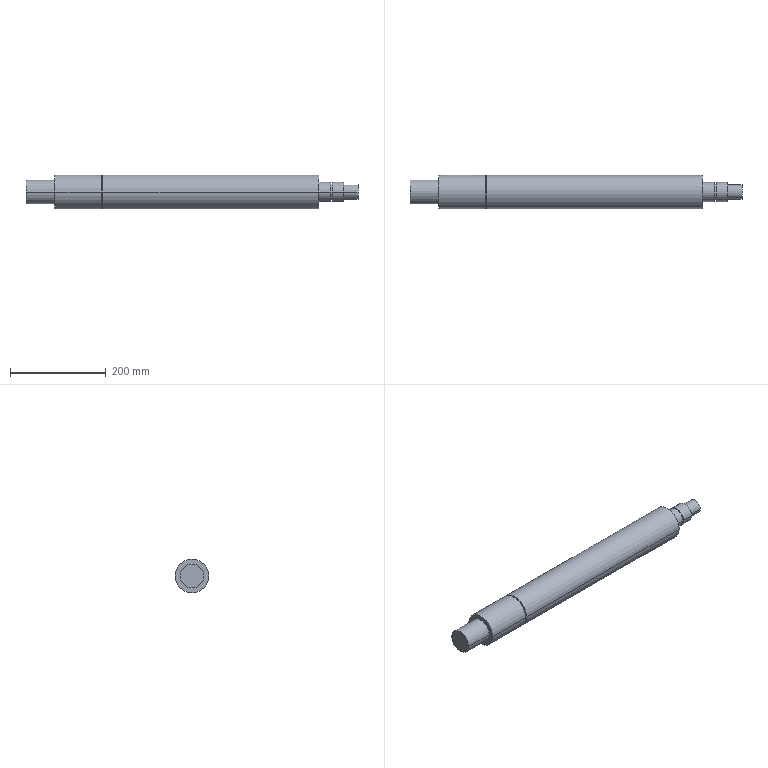Part | SolidWorks | features ICE 1, Revolution 1 | 1 solid | 30 faces | box 691.99 x 70 x 70 mm | volume 2315644 mm3 | cylinder 18 | plane 12 | commonest cylinder face diameters 40 x4 70 x4 12 x2 30 x2 34.7 x2 50 x2
STEP:
#1=CARTESIAN_POINT('',(691.99,-15.,0.));
#2=VERTEX_POINT('',#1);
#3=CARTESIAN_POINT('',(691.99,15.,0.));
#4=VERTEX_POINT('',#3);
#5=CARTESIAN_POINT('',(691.99,0.,0.));
#6=DIRECTION('',(-1.,0.,0.));
#7=DIRECTION('',(0.,-1.,0.));
#8=AXIS2_PLACEMENT_3D('',#5,#6,#7);
#9=CIRCLE('',#8,15.);
#10=EDGE_CURVE('',#2,#4,#9,.T.);
#11=ORIENTED_EDGE('',*,*,#10,.T.);
#12=CARTESIAN_POINT('',(661.99,15.,0.));
#13=VERTEX_POINT('',#12);
#14=CARTESIAN_POINT('',(0.,15.,0.));
#15=DIRECTION('',(-1.,0.,0.));
#16=VECTOR('',#15,1000.);
#17=LINE('',#14,#16);
#18=EDGE_CURVE('',#4,#13,#17,.T.);
#19=ORIENTED_EDGE('',*,*,#18,.T.);
#20=CARTESIAN_POINT('',(661.99,-15.,0.));
#21=VERTEX_POINT('',#20);
#22=CARTESIAN_POINT('',(661.99,0.,0.));
#23=DIRECTION('',(-1.,0.,0.));
#24=DIRECTION('',(0.,-1.,0.));
#25=AXIS2_PLACEMENT_3D('',#22,#23,#24);
#26=CIRCLE('',#25,15.);
#27=EDGE_CURVE('',#21,#13,#26,.T.);
#28=ORIENTED_EDGE('',*,*,#27,.F.);
#29=CARTESIAN_POINT('',(0.,-15.,0.));
#30=DIRECTION('',(-1.,0.,0.));
#31=VECTOR('',#30,1000.);
#32=LINE('',#29,#31);
#33=EDGE_CURVE('',#2,#21,#32,.T.);
#34=ORIENTED_EDGE('',*,*,#33,.F.);
#35=EDGE_LOOP('',(#11,#19,#28,#34));
#36=FACE_OUTER_BOUND('',#35,.T.);
#37=CARTESIAN_POINT('',(0.,0.,0.));
#38=DIRECTION('',(-1.,0.,0.));
#39=DIRECTION('',(0.,-1.,0.));
#40=AXIS2_PLACEMENT_3D('',#37,#38,#39);
#41=CYLINDRICAL_SURFACE('',#40,15.);
#42=ADVANCED_FACE('',(#36),#41,.T.);
#43=CARTESIAN_POINT('',(661.99,-20.,0.));
#44=VERTEX_POINT('',#43);
#45=CARTESIAN_POINT('',(661.99,20.,0.));
#46=VERTEX_POINT('',#45);
#47=CARTESIAN_POINT('',(661.99,0.,0.));
#48=DIRECTION('',(-1.,0.,0.));
#49=DIRECTION('',(0.,-1.,0.));
#50=AXIS2_PLACEMENT_3D('',#47,#48,#49);
#51=CIRCLE('',#50,20.);
#52=EDGE_CURVE('',#44,#46,#51,.T.);
#53=ORIENTED_EDGE('',*,*,#52,.T.);
#54=CARTESIAN_POINT('',(638.32,20.,0.));
#55=VERTEX_POINT('',#54);
#56=CARTESIAN_POINT('',(0.,20.,0.));
#57=DIRECTION('',(-1.,0.,0.));
#58=VECTOR('',#57,1000.);
#59=LINE('',#56,#58);
#60=EDGE_CURVE('',#46,#55,#59,.T.);
#61=ORIENTED_EDGE('',*,*,#60,.T.);
#62=CARTESIAN_POINT('',(638.32,-20.,0.));
#63=VERTEX_POINT('',#62);
#64=CARTESIAN_POINT('',(638.32,0.,0.));
#65=DIRECTION('',(-1.,0.,0.));
#66=DIRECTION('',(0.,-1.,0.));
#67=AXIS2_PLACEMENT_3D('',#64,#65,#66);
#68=CIRCLE('',#67,20.);
#69=EDGE_CURVE('',#63,#55,#68,.T.);
#70=ORIENTED_EDGE('',*,*,#69,.F.);
#71=CARTESIAN_POINT('',(0.,-20.,0.));
#72=DIRECTION('',(-1.,0.,0.));
#73=VECTOR('',#72,1000.);
#74=LINE('',#71,#73);
#75=EDGE_CURVE('',#44,#63,#74,.T.);
#76=ORIENTED_EDGE('',*,*,#75,.F.);
#77=EDGE_LOOP('',(#53,#61,#70,#76));
#78=FACE_OUTER_BOUND('',#77,.T.);
#79=CARTESIAN_POINT('',(0.,0.,0.));
#80=DIRECTION('',(-1.,0.,0.));
#81=DIRECTION('',(0.,-1.,0.));
#82=AXIS2_PLACEMENT_3D('',#79,#80,#81);
#83=CYLINDRICAL_SURFACE('',#82,20.);
#84=ADVANCED_FACE('',(#78),#83,.T.);
#85=CARTESIAN_POINT('',(638.32,-17.35,0.));
#86=VERTEX_POINT('',#85);
#87=CARTESIAN_POINT('',(638.32,17.35,0.));
#88=VERTEX_POINT('',#87);
#89=CARTESIAN_POINT('',(638.32,0.,0.));
#90=DIRECTION('',(-1.,0.,0.));
#91=DIRECTION('',(0.,-1.,0.));
#92=AXIS2_PLACEMENT_3D('',#89,#90,#91);
#93=CIRCLE('',#92,17.35);
#94=EDGE_CURVE('',#86,#88,#93,.T.);
#95=ORIENTED_EDGE('',*,*,#94,.T.);
#96=CARTESIAN_POINT('',(635.67,17.35,0.));
#97=VERTEX_POINT('',#96);
#98=CARTESIAN_POINT('',(0.,17.35,0.));
#99=DIRECTION('',(-1.,0.,0.));
#100=VECTOR('',#99,1000.);
#101=LINE('',#98,#100);
#102=EDGE_CURVE('',#88,#97,#101,.T.);
#103=ORIENTED_EDGE('',*,*,#102,.T.);
#104=CARTESIAN_POINT('',(635.67,-17.35,0.));
#105=VERTEX_POINT('',#104);
#106=CARTESIAN_POINT('',(635.67,0.,0.));
#107=DIRECTION('',(-1.,0.,0.));
#108=DIRECTION('',(0.,-1.,0.));
#109=AXIS2_PLACEMENT_3D('',#106,#107,#108);
#110=CIRCLE('',#109,17.35);
#111=EDGE_CURVE('',#105,#97,#110,.T.);
#112=ORIENTED_EDGE('',*,*,#111,.F.);
#113=CARTESIAN_POINT('',(0.,-17.35,0.));
#114=DIRECTION('',(-1.,0.,0.));
#115=VECTOR('',#114,1000.);
#116=LINE('',#113,#115);
#117=EDGE_CURVE('',#86,#105,#116,.T.);
#118=ORIENTED_EDGE('',*,*,#117,.F.);
#119=EDGE_LOOP('',(#95,#103,#112,#118));
#120=FACE_OUTER_BOUND('',#119,.T.);
#121=CARTESIAN_POINT('',(0.,0.,0.));
#122=DIRECTION('',(-1.,0.,0.));
#123=DIRECTION('',(0.,-1.,0.));
#124=AXIS2_PLACEMENT_3D('',#121,#122,#123);
#125=CYLINDRICAL_SURFACE('',#124,17.35);
#126=ADVANCED_FACE('',(#120),#125,.T.);
#127=CARTESIAN_POINT('',(635.67,-20.,0.));
#128=VERTEX_POINT('',#127);
#129=CARTESIAN_POINT('',(635.67,20.,0.));
#130=VERTEX_POINT('',#129);
#131=CARTESIAN_POINT('',(635.67,0.,0.));
#132=DIRECTION('',(-1.,0.,0.));
#133=DIRECTION('',(0.,-1.,0.));
#134=AXIS2_PLACEMENT_3D('',#131,#132,#133);
#135=CIRCLE('',#134,20.);
#136=EDGE_CURVE('',#128,#130,#135,.T.);
#137=ORIENTED_EDGE('',*,*,#136,.T.);
#138=CARTESIAN_POINT('',(610.,20.,0.));
#139=VERTEX_POINT('',#138);
#140=CARTESIAN_POINT('',(0.,20.,0.));
#141=DIRECTION('',(-1.,0.,0.));
#142=VECTOR('',#141,1000.);
#143=LINE('',#140,#142);
#144=EDGE_CURVE('',#130,#139,#143,.T.);
#145=ORIENTED_EDGE('',*,*,#144,.T.);
#146=CARTESIAN_POINT('',(610.,-20.,0.));
#147=VERTEX_POINT('',#146);
#148=CARTESIAN_POINT('',(610.,0.,0.));
#149=DIRECTION('',(-1.,0.,0.));
#150=DIRECTION('',(0.,-1.,0.));
#151=AXIS2_PLACEMENT_3D('',#148,#149,#150);
#152=CIRCLE('',#151,20.);
#153=EDGE_CURVE('',#147,#139,#152,.T.);
#154=ORIENTED_EDGE('',*,*,#153,.F.);
#155=CARTESIAN_POINT('',(0.,-20.,0.));
#156=DIRECTION('',(-1.,0.,0.));
#157=VECTOR('',#156,1000.);
#158=LINE('',#155,#157);
#159=EDGE_CURVE('',#128,#147,#158,.T.);
#160=ORIENTED_EDGE('',*,*,#159,.F.);
#161=EDGE_LOOP('',(#137,#145,#154,#160));
#162=FACE_OUTER_BOUND('',#161,.T.);
#163=CARTESIAN_POINT('',(0.,0.,0.));
#164=DIRECTION('',(-1.,0.,0.));
#165=DIRECTION('',(0.,-1.,0.));
#166=AXIS2_PLACEMENT_3D('',#163,#164,#165);
#167=CYLINDRICAL_SURFACE('',#166,20.);
#168=ADVANCED_FACE('',(#162),#167,.T.);
#169=CARTESIAN_POINT('',(610.,-35.,0.));
#170=VERTEX_POINT('',#169);
#171=CARTESIAN_POINT('',(610.,35.,0.));
#172=VERTEX_POINT('',#171);
#173=CARTESIAN_POINT('',(610.,0.,0.));
#174=DIRECTION('',(-1.,0.,0.));
#175=DIRECTION('',(0.,-1.,0.));
#176=AXIS2_PLACEMENT_3D('',#173,#174,#175);
#177=CIRCLE('',#176,35.);
#178=EDGE_CURVE('',#170,#172,#177,.T.);
#179=ORIENTED_EDGE('',*,*,#178,.T.);
#180=CARTESIAN_POINT('',(160.,35.,0.));
#181=VERTEX_POINT('',#180);
#182=CARTESIAN_POINT('',(0.,35.,0.));
#183=DIRECTION('',(-1.,0.,0.));
#184=VECTOR('',#183,1000.);
#185=LINE('',#182,#184);
#186=EDGE_CURVE('',#172,#181,#185,.T.);
#187=ORIENTED_EDGE('',*,*,#186,.T.);
#188=CARTESIAN_POINT('',(160.,-35.,0.));
#189=VERTEX_POINT('',#188);
#190=CARTESIAN_POINT('',(160.,0.,0.));
#191=DIRECTION('',(-1.,0.,0.));
#192=DIRECTION('',(0.,-1.,0.));
#193=AXIS2_PLACEMENT_3D('',#190,#191,#192);
#194=CIRCLE('',#193,35.);
#195=EDGE_CURVE('',#189,#181,#194,.T.);
#196=ORIENTED_EDGE('',*,*,#195,.F.);
#197=CARTESIAN_POINT('',(0.,-35.,0.));
#198=DIRECTION('',(-1.,0.,0.));
#199=VECTOR('',#198,1000.);
#200=LINE('',#197,#199);
#201=EDGE_CURVE('',#170,#189,#200,.T.);
#202=ORIENTED_EDGE('',*,*,#201,.F.);
#203=EDGE_LOOP('',(#179,#187,#196,#202));
#204=FACE_OUTER_BOUND('',#203,.T.);
#205=CARTESIAN_POINT('',(0.,0.,0.));
#206=DIRECTION('',(-1.,0.,0.));
#207=DIRECTION('',(0.,-1.,0.));
#208=AXIS2_PLACEMENT_3D('',#205,#206,#207);
#209=CYLINDRICAL_SURFACE('',#208,35.);
#210=ADVANCED_FACE('',(#204),#209,.T.);
#211=CARTESIAN_POINT('',(160.,-32.35,0.));
#212=VERTEX_POINT('',#211);
#213=CARTESIAN_POINT('',(160.,32.35,0.));
#214=VERTEX_POINT('',#213);
#215=CARTESIAN_POINT('',(160.,0.,0.));
#216=DIRECTION('',(-1.,0.,0.));
#217=DIRECTION('',(0.,-1.,0.));
#218=AXIS2_PLACEMENT_3D('',#215,#216,#217);
#219=CIRCLE('',#218,32.35);
#220=EDGE_CURVE('',#212,#214,#219,.T.);
#221=ORIENTED_EDGE('',*,*,#220,.T.);
#222=CARTESIAN_POINT('',(157.35,32.35,0.));
#223=VERTEX_POINT('',#222);
#224=CARTESIAN_POINT('',(0.,32.35,0.));
#225=DIRECTION('',(-1.,0.,0.));
#226=VECTOR('',#225,1000.);
#227=LINE('',#224,#226);
#228=EDGE_CURVE('',#214,#223,#227,.T.);
#229=ORIENTED_EDGE('',*,*,#228,.T.);
#230=CARTESIAN_POINT('',(157.35,-32.35,0.));
#231=VERTEX_POINT('',#230);
#232=CARTESIAN_POINT('',(157.35,0.,0.));
#233=DIRECTION('',(-1.,0.,0.));
#234=DIRECTION('',(0.,-1.,0.));
#235=AXIS2_PLACEMENT_3D('',#232,#233,#234);
#236=CIRCLE('',#235,32.35);
#237=EDGE_CURVE('',#231,#223,#236,.T.);
#238=ORIENTED_EDGE('',*,*,#237,.F.);
#239=CARTESIAN_POINT('',(0.,-32.35,0.));
#240=DIRECTION('',(-1.,0.,0.));
#241=VECTOR('',#240,1000.);
#242=LINE('',#239,#241);
#243=EDGE_CURVE('',#212,#231,#242,.T.);
#244=ORIENTED_EDGE('',*,*,#243,.F.);
#245=EDGE_LOOP('',(#221,#229,#238,#244));
#246=FACE_OUTER_BOUND('',#245,.T.);
#247=CARTESIAN_POINT('',(0.,0.,0.));
#248=DIRECTION('',(-1.,0.,0.));
#249=DIRECTION('',(0.,-1.,0.));
#250=AXIS2_PLACEMENT_3D('',#247,#248,#249);
#251=CYLINDRICAL_SURFACE('',#250,32.35);
#252=ADVANCED_FACE('',(#246),#251,.T.);
#253=CARTESIAN_POINT('',(60.,-25.,0.));
#254=VERTEX_POINT('',#253);
#255=CARTESIAN_POINT('',(60.,25.,0.));
#256=VERTEX_POINT('',#255);
#257=CARTESIAN_POINT('',(60.,0.,0.));
#258=DIRECTION('',(-1.,0.,0.));
#259=DIRECTION('',(0.,-1.,0.));
#260=AXIS2_PLACEMENT_3D('',#257,#258,#259);
#261=CIRCLE('',#260,25.);
#262=EDGE_CURVE('',#254,#256,#261,.T.);
#263=ORIENTED_EDGE('',*,*,#262,.T.);
#264=CARTESIAN_POINT('',(0.,25.,0.));
#265=VERTEX_POINT('',#264);
#266=CARTESIAN_POINT('',(0.,25.,0.));
#267=DIRECTION('',(-1.,0.,0.));
#268=VECTOR('',#267,1000.);
#269=LINE('',#266,#268);
#270=EDGE_CURVE('',#256,#265,#269,.T.);
#271=ORIENTED_EDGE('',*,*,#270,.T.);
#272=CARTESIAN_POINT('',(0.,-25.,0.));
#273=VERTEX_POINT('',#272);
#274=CARTESIAN_POINT('',(0.,0.,0.));
#275=DIRECTION('',(-1.,0.,0.));
#276=DIRECTION('',(0.,-1.,0.));
#277=AXIS2_PLACEMENT_3D('',#274,#275,#276);
#278=CIRCLE('',#277,25.);
#279=EDGE_CURVE('',#273,#265,#278,.T.);
#280=ORIENTED_EDGE('',*,*,#279,.F.);
#281=CARTESIAN_POINT('',(0.,-25.,0.));
#282=DIRECTION('',(-1.,0.,0.));
#283=VECTOR('',#282,1000.);
#284=LINE('',#281,#283);
#285=EDGE_CURVE('',#254,#273,#284,.T.);
#286=ORIENTED_EDGE('',*,*,#285,.F.);
#287=EDGE_LOOP('',(#263,#271,#280,#286));
#288=FACE_OUTER_BOUND('',#287,.T.);
#289=CARTESIAN_POINT('',(0.,0.,0.));
#290=DIRECTION('',(-1.,0.,0.));
#291=DIRECTION('',(0.,-1.,0.));
#292=AXIS2_PLACEMENT_3D('',#289,#290,#291);
#293=CYLINDRICAL_SURFACE('',#292,25.);
#294=ADVANCED_FACE('',(#288),#293,.T.);
#295=CARTESIAN_POINT('',(157.35,-35.,0.));
#296=VERTEX_POINT('',#295);
#297=CARTESIAN_POINT('',(157.35,35.,0.));
#298=VERTEX_POINT('',#297);
#299=CARTESIAN_POINT('',(157.35,0.,0.));
#300=DIRECTION('',(-1.,0.,0.));
#301=DIRECTION('',(0.,-1.,0.));
#302=AXIS2_PLACEMENT_3D('',#299,#300,#301);
#303=CIRCLE('',#302,35.);
#304=EDGE_CURVE('',#296,#298,#303,.T.);
#305=ORIENTED_EDGE('',*,*,#304,.T.);
#306=CARTESIAN_POINT('',(130.,35.,0.));
#307=VERTEX_POINT('',#306);
#308=CARTESIAN_POINT('',(0.,35.,0.));
#309=DIRECTION('',(-1.,0.,0.));
#310=VECTOR('',#309,1000.);
#311=LINE('',#308,#310);
#312=EDGE_CURVE('',#298,#307,#311,.T.);
#313=ORIENTED_EDGE('',*,*,#312,.T.);
#314=CARTESIAN_POINT('',(124.,34.482,6.));
#315=VERTEX_POINT('',#314);
#316=CARTESIAN_POINT('',(124.,34.482,6.));
#317=CARTESIAN_POINT('',(124.397,34.482,6.));
#318=CARTESIAN_POINT('',(124.788,34.489,5.961));
#319=CARTESIAN_POINT('',(125.364,34.508,5.846));
#320=CARTESIAN_POINT('',(125.554,34.516,5.799));
#321=CARTESIAN_POINT('',(125.932,34.535,5.684));
#322=CARTESIAN_POINT('',(126.119,34.546,5.617));
#323=CARTESIAN_POINT('',(126.664,34.583,5.391));
#324=CARTESIAN_POINT('',(127.008,34.611,5.206));
#325=CARTESIAN_POINT('',(127.66,34.674,4.77));
#326=CARTESIAN_POINT('',(127.968,34.708,4.517));
#327=CARTESIAN_POINT('',(128.521,34.776,3.965));
#328=CARTESIAN_POINT('',(128.769,34.809,3.663));
#329=CARTESIAN_POINT('',(129.207,34.872,3.007));
#330=CARTESIAN_POINT('',(129.393,34.901,2.659));
#331=CARTESIAN_POINT('',(129.618,34.936,2.117));
#332=CARTESIAN_POINT('',(129.684,34.947,1.933));
#333=CARTESIAN_POINT('',(129.798,34.966,1.557));
#334=CARTESIAN_POINT('',(129.846,34.974,1.364));
#335=CARTESIAN_POINT('',(129.962,34.993,0.7822));
#336=CARTESIAN_POINT('',(130.,35.,0.3923));
#337=CARTESIAN_POINT('',(130.,35.,0.));
#338=B_SPLINE_CURVE_WITH_KNOTS('',3,(#316,#317,#318,#319,#320,#321,#322,#323,#324,#325,#326,#327,#328,#329,#330,#331,#332,#333,#334,#335,#336,#337),.UNSPECIFIED.,.F.,.F.,(4,2,2,2,2,2,2,2,2,2,4),(0.,0.001175,0.001762,0.00235,0.003525,0.004699,0.005874,0.007049,0.007637,0.008224,0.009399),.UNSPECIFIED.);
#339=EDGE_CURVE('',#315,#307,#338,.T.);
#340=ORIENTED_EDGE('',*,*,#339,.F.);
#341=CARTESIAN_POINT('',(81.,34.482,6.));
#342=VERTEX_POINT('',#341);
#343=CARTESIAN_POINT('',(0.,34.482,6.));
#344=DIRECTION('',(1.,0.,0.));
#345=VECTOR('',#344,1000.);
#346=LINE('',#343,#345);
#347=EDGE_CURVE('',#342,#315,#346,.T.);
#348=ORIENTED_EDGE('',*,*,#347,.F.);
#349=CARTESIAN_POINT('',(75.,35.,0.));
#350=VERTEX_POINT('',#349);
#351=CARTESIAN_POINT('',(75.,35.,0.));
#352=CARTESIAN_POINT('',(75.,35.,0.3919));
#353=CARTESIAN_POINT('',(75.039,34.993,0.79));
#354=CARTESIAN_POINT('',(75.193,34.967,1.559));
#355=CARTESIAN_POINT('',(75.306,34.948,1.934));
#356=CARTESIAN_POINT('',(75.532,34.913,2.479));
#357=CARTESIAN_POINT('',(75.617,34.899,2.658));
#358=CARTESIAN_POINT('',(75.803,34.871,3.005));
#359=CARTESIAN_POINT('',(75.904,34.856,3.173));
#360=CARTESIAN_POINT('',(76.229,34.81,3.659));
#361=CARTESIAN_POINT('',(76.478,34.776,3.963));
#362=CARTESIAN_POINT('',(77.036,34.708,4.521));
#363=CARTESIAN_POINT('',(77.338,34.674,4.769));
#364=CARTESIAN_POINT('',(77.824,34.627,5.094));
#365=CARTESIAN_POINT('',(77.992,34.612,5.195));
#366=CARTESIAN_POINT('',(78.339,34.584,5.381));
#367=CARTESIAN_POINT('',(78.518,34.571,5.466));
#368=CARTESIAN_POINT('',(79.062,34.534,5.692));
#369=CARTESIAN_POINT('',(79.436,34.515,5.806));
#370=CARTESIAN_POINT('',(80.206,34.489,5.96));
#371=CARTESIAN_POINT('',(80.603,34.482,6.));
#372=CARTESIAN_POINT('',(81.,34.482,6.));
#373=B_SPLINE_CURVE_WITH_KNOTS('',3,(#351,#352,#353,#354,#355,#356,#357,#358,#359,#360,#361,#362,#363,#364,#365,#366,#367,#368,#369,#370,#371,#372),.UNSPECIFIED.,.F.,.F.,(4,2,2,2,2,2,2,2,2,2,4),(0.009399,0.01057,0.01175,0.01233,0.01292,0.01409,0.01527,0.01585,0.01644,0.01761,0.01879),.UNSPECIFIED.);
#374=EDGE_CURVE('',#350,#342,#373,.T.);
#375=ORIENTED_EDGE('',*,*,#374,.F.);
#376=CARTESIAN_POINT('',(60.,35.,0.));
#377=VERTEX_POINT('',#376);
#378=CARTESIAN_POINT('',(0.,35.,0.));
#379=DIRECTION('',(-1.,0.,0.));
#380=VECTOR('',#379,1000.);
#381=LINE('',#378,#380);
#382=EDGE_CURVE('',#350,#377,#381,.T.);
#383=ORIENTED_EDGE('',*,*,#382,.T.);
#384=CARTESIAN_POINT('',(60.,-35.,0.));
#385=VERTEX_POINT('',#384);
#386=CARTESIAN_POINT('',(60.,0.,0.));
#387=DIRECTION('',(-1.,0.,0.));
#388=DIRECTION('',(0.,-1.,0.));
#389=AXIS2_PLACEMENT_3D('',#386,#387,#388);
#390=CIRCLE('',#389,35.);
#391=EDGE_CURVE('',#385,#377,#390,.T.);
#392=ORIENTED_EDGE('',*,*,#391,.F.);
#393=CARTESIAN_POINT('',(0.,-35.,0.));
#394=DIRECTION('',(-1.,0.,0.));
#395=VECTOR('',#394,1000.);
#396=LINE('',#393,#395);
#397=EDGE_CURVE('',#296,#385,#396,.T.);
#398=ORIENTED_EDGE('',*,*,#397,.F.);
#399=EDGE_LOOP('',(#305,#313,#340,#348,#375,#383,#392,#398));
#400=FACE_OUTER_BOUND('',#399,.T.);
#401=CARTESIAN_POINT('',(0.,0.,0.));
#402=DIRECTION('',(-1.,0.,0.));
#403=DIRECTION('',(0.,-1.,0.));
#404=AXIS2_PLACEMENT_3D('',#401,#402,#403);
#405=CYLINDRICAL_SURFACE('',#404,35.);
#406=ADVANCED_FACE('',(#400),#405,.T.);
#407=ORIENTED_EDGE('',*,*,#312,.F.);
#408=CARTESIAN_POINT('',(157.35,0.,0.));
#409=DIRECTION('',(-1.,0.,0.));
#410=DIRECTION('',(0.,-1.,0.));
#411=AXIS2_PLACEMENT_3D('',#408,#409,#410);
#412=CIRCLE('',#411,35.);
#413=EDGE_CURVE('',#298,#296,#412,.T.);
#414=ORIENTED_EDGE('',*,*,#413,.T.);
#415=ORIENTED_EDGE('',*,*,#397,.T.);
#416=CARTESIAN_POINT('',(60.,0.,0.));
#417=DIRECTION('',(-1.,0.,0.));
#418=DIRECTION('',(0.,-1.,0.));
#419=AXIS2_PLACEMENT_3D('',#416,#417,#418);
#420=CIRCLE('',#419,35.);
#421=EDGE_CURVE('',#377,#385,#420,.T.);
#422=ORIENTED_EDGE('',*,*,#421,.F.);
#423=ORIENTED_EDGE('',*,*,#382,.F.);
#424=CARTESIAN_POINT('',(81.,34.482,-6.));
#425=VERTEX_POINT('',#424);
#426=CARTESIAN_POINT('',(81.,34.482,-6.));
#427=CARTESIAN_POINT('',(80.603,34.482,-6.));
#428=CARTESIAN_POINT('',(80.212,34.489,-5.961));
#429=CARTESIAN_POINT('',(79.636,34.508,-5.846));
#430=CARTESIAN_POINT('',(79.446,34.516,-5.799));
#431=CARTESIAN_POINT('',(79.068,34.535,-5.684));
#432=CARTESIAN_POINT('',(78.881,34.546,-5.617));
#433=CARTESIAN_POINT('',(78.336,34.583,-5.391));
#434=CARTESIAN_POINT('',(77.992,34.611,-5.206));
#435=CARTESIAN_POINT('',(77.34,34.674,-4.77));
#436=CARTESIAN_POINT('',(77.032,34.708,-4.517));
#437=CARTESIAN_POINT('',(76.479,34.776,-3.965));
#438=CARTESIAN_POINT('',(76.231,34.809,-3.663));
#439=CARTESIAN_POINT('',(75.793,34.872,-3.007));
#440=CARTESIAN_POINT('',(75.607,34.901,-2.659));
#441=CARTESIAN_POINT('',(75.382,34.936,-2.117));
#442=CARTESIAN_POINT('',(75.316,34.947,-1.933));
#443=CARTESIAN_POINT('',(75.202,34.966,-1.557));
#444=CARTESIAN_POINT('',(75.154,34.974,-1.364));
#445=CARTESIAN_POINT('',(75.038,34.993,-0.7822));
#446=CARTESIAN_POINT('',(75.,35.,-0.3923));
#447=CARTESIAN_POINT('',(75.,35.,0.));
#448=B_SPLINE_CURVE_WITH_KNOTS('',3,(#426,#427,#428,#429,#430,#431,#432,#433,#434,#435,#436,#437,#438,#439,#440,#441,#442,#443,#444,#445,#446,#447),.UNSPECIFIED.,.F.,.F.,(4,2,2,2,2,2,2,2,2,2,4),(0.,0.001175,0.001762,0.00235,0.003525,0.004699,0.005874,0.007049,0.007637,0.008224,0.009399),.UNSPECIFIED.);
#449=EDGE_CURVE('',#425,#350,#448,.T.);
#450=ORIENTED_EDGE('',*,*,#449,.F.);
#451=CARTESIAN_POINT('',(124.,34.482,-6.));
#452=VERTEX_POINT('',#451);
#453=CARTESIAN_POINT('',(0.,34.482,-6.));
#454=DIRECTION('',(-1.,0.,0.));
#455=VECTOR('',#454,1000.);
#456=LINE('',#453,#455);
#457=EDGE_CURVE('',#452,#425,#456,.T.);
#458=ORIENTED_EDGE('',*,*,#457,.F.);
#459=CARTESIAN_POINT('',(130.,35.,0.));
#460=CARTESIAN_POINT('',(130.,35.,-0.3919));
#461=CARTESIAN_POINT('',(129.961,34.993,-0.79));
#462=CARTESIAN_POINT('',(129.807,34.967,-1.559));
#463=CARTESIAN_POINT('',(129.694,34.948,-1.934));
#464=CARTESIAN_POINT('',(129.468,34.913,-2.479));
#465=CARTESIAN_POINT('',(129.383,34.899,-2.658));
#466=CARTESIAN_POINT('',(129.197,34.871,-3.005));
#467=CARTESIAN_POINT('',(129.096,34.856,-3.173));
#468=CARTESIAN_POINT('',(128.771,34.81,-3.659));
#469=CARTESIAN_POINT('',(128.522,34.776,-3.963));
#470=CARTESIAN_POINT('',(127.964,34.708,-4.521));
#471=CARTESIAN_POINT('',(127.662,34.674,-4.769));
#472=CARTESIAN_POINT('',(127.176,34.627,-5.094));
#473=CARTESIAN_POINT('',(127.008,34.612,-5.195));
#474=CARTESIAN_POINT('',(126.661,34.584,-5.381));
#475=CARTESIAN_POINT('',(126.482,34.571,-5.466));
#476=CARTESIAN_POINT('',(125.938,34.534,-5.692));
#477=CARTESIAN_POINT('',(125.564,34.515,-5.806));
#478=CARTESIAN_POINT('',(124.794,34.489,-5.96));
#479=CARTESIAN_POINT('',(124.397,34.482,-6.));
#480=CARTESIAN_POINT('',(124.,34.482,-6.));
#481=B_SPLINE_CURVE_WITH_KNOTS('',3,(#459,#460,#461,#462,#463,#464,#465,#466,#467,#468,#469,#470,#471,#472,#473,#474,#475,#476,#477,#478,#479,#480),.UNSPECIFIED.,.F.,.F.,(4,2,2,2,2,2,2,2,2,2,4),(0.009399,0.01057,0.01175,0.01233,0.01292,0.01409,0.01527,0.01585,0.01644,0.01761,0.01879),.UNSPECIFIED.);
#482=EDGE_CURVE('',#307,#452,#481,.T.);
#483=ORIENTED_EDGE('',*,*,#482,.F.);
#484=EDGE_LOOP('',(#407,#414,#415,#422,#423,#450,#458,#483));
#485=FACE_OUTER_BOUND('',#484,.T.);
#486=CARTESIAN_POINT('',(0.,0.,0.));
#487=DIRECTION('',(-1.,0.,0.));
#488=DIRECTION('',(0.,-1.,0.));
#489=AXIS2_PLACEMENT_3D('',#486,#487,#488);
#490=CYLINDRICAL_SURFACE('',#489,35.);
#491=ADVANCED_FACE('',(#485),#490,.T.);
#492=ORIENTED_EDGE('',*,*,#279,.T.);
#493=CARTESIAN_POINT('',(0.,0.,0.));
#494=DIRECTION('',(-1.,0.,0.));
#495=DIRECTION('',(0.,-1.,0.));
#496=AXIS2_PLACEMENT_3D('',#493,#494,#495);
#497=CIRCLE('',#496,25.);
#498=EDGE_CURVE('',#265,#273,#497,.T.);
#499=ORIENTED_EDGE('',*,*,#498,.T.);
#500=EDGE_LOOP('',(#492,#499));
#501=FACE_OUTER_BOUND('',#500,.T.);
#502=CARTESIAN_POINT('',(0.,0.,0.));
#503=DIRECTION('',(1.,0.,0.));
#504=DIRECTION('',(0.,1.,0.));
#505=AXIS2_PLACEMENT_3D('',#502,#503,#504);
#506=PLANE('',#505);
#507=ADVANCED_FACE('',(#501),#506,.F.);
#508=ORIENTED_EDGE('',*,*,#270,.F.);
#509=CARTESIAN_POINT('',(60.,0.,0.));
#510=DIRECTION('',(-1.,0.,0.));
#511=DIRECTION('',(0.,-1.,0.));
#512=AXIS2_PLACEMENT_3D('',#509,#510,#511);
#513=CIRCLE('',#512,25.);
#514=EDGE_CURVE('',#256,#254,#513,.T.);
#515=ORIENTED_EDGE('',*,*,#514,.T.);
#516=ORIENTED_EDGE('',*,*,#285,.T.);
#517=ORIENTED_EDGE('',*,*,#498,.F.);
#518=EDGE_LOOP('',(#508,#515,#516,#517));
#519=FACE_OUTER_BOUND('',#518,.T.);
#520=CARTESIAN_POINT('',(0.,0.,0.));
#521=DIRECTION('',(-1.,0.,0.));
#522=DIRECTION('',(0.,-1.,0.));
#523=AXIS2_PLACEMENT_3D('',#520,#521,#522);
#524=CYLINDRICAL_SURFACE('',#523,25.);
#525=ADVANCED_FACE('',(#519),#524,.T.);
#526=ORIENTED_EDGE('',*,*,#262,.F.);
#527=ORIENTED_EDGE('',*,*,#514,.F.);
#528=EDGE_LOOP('',(#526,#527));
#529=FACE_BOUND('',#528,.T.);
#530=ORIENTED_EDGE('',*,*,#391,.T.);
#531=ORIENTED_EDGE('',*,*,#421,.T.);
#532=EDGE_LOOP('',(#530,#531));
#533=FACE_OUTER_BOUND('',#532,.T.);
#534=CARTESIAN_POINT('',(60.,25.,0.));
#535=DIRECTION('',(1.,0.,0.));
#536=DIRECTION('',(0.,1.,0.));
#537=AXIS2_PLACEMENT_3D('',#534,#535,#536);
#538=PLANE('',#537);
#539=ADVANCED_FACE('',(#529,#533),#538,.F.);
#540=ORIENTED_EDGE('',*,*,#304,.F.);
#541=ORIENTED_EDGE('',*,*,#413,.F.);
#542=EDGE_LOOP('',(#540,#541));
#543=FACE_OUTER_BOUND('',#542,.T.);
#544=ORIENTED_EDGE('',*,*,#237,.T.);
#545=CARTESIAN_POINT('',(157.35,0.,0.));
#546=DIRECTION('',(-1.,0.,0.));
#547=DIRECTION('',(0.,-1.,0.));
#548=AXIS2_PLACEMENT_3D('',#545,#546,#547);
#549=CIRCLE('',#548,32.35);
#550=EDGE_CURVE('',#223,#231,#549,.T.);
#551=ORIENTED_EDGE('',*,*,#550,.T.);
#552=EDGE_LOOP('',(#544,#551));
#553=FACE_BOUND('',#552,.T.);
#554=CARTESIAN_POINT('',(157.35,35.,0.));
#555=DIRECTION('',(-1.,0.,0.));
#556=DIRECTION('',(0.,-1.,0.));
#557=AXIS2_PLACEMENT_3D('',#554,#555,#556);
#558=PLANE('',#557);
#559=ADVANCED_FACE('',(#543,#553),#558,.F.);
#560=ORIENTED_EDGE('',*,*,#228,.F.);
#561=CARTESIAN_POINT('',(160.,0.,0.));
#562=DIRECTION('',(-1.,0.,0.));
#563=DIRECTION('',(0.,-1.,0.));
#564=AXIS2_PLACEMENT_3D('',#561,#562,#563);
#565=CIRCLE('',#564,32.35);
#566=EDGE_CURVE('',#214,#212,#565,.T.);
#567=ORIENTED_EDGE('',*,*,#566,.T.);
#568=ORIENTED_EDGE('',*,*,#243,.T.);
#569=ORIENTED_EDGE('',*,*,#550,.F.);
#570=EDGE_LOOP('',(#560,#567,#568,#569));
#571=FACE_OUTER_BOUND('',#570,.T.);
#572=CARTESIAN_POINT('',(0.,0.,0.));
#573=DIRECTION('',(-1.,0.,0.));
#574=DIRECTION('',(0.,-1.,0.));
#575=AXIS2_PLACEMENT_3D('',#572,#573,#574);
#576=CYLINDRICAL_SURFACE('',#575,32.35);
#577=ADVANCED_FACE('',(#571),#576,.T.);
#578=ORIENTED_EDGE('',*,*,#220,.F.);
#579=ORIENTED_EDGE('',*,*,#566,.F.);
#580=EDGE_LOOP('',(#578,#579));
#581=FACE_BOUND('',#580,.T.);
#582=ORIENTED_EDGE('',*,*,#195,.T.);
#583=CARTESIAN_POINT('',(160.,0.,0.));
#584=DIRECTION('',(-1.,0.,0.));
#585=DIRECTION('',(0.,-1.,0.));
#586=AXIS2_PLACEMENT_3D('',#583,#584,#585);
#587=CIRCLE('',#586,35.);
#588=EDGE_CURVE('',#181,#189,#587,.T.);
#589=ORIENTED_EDGE('',*,*,#588,.T.);
#590=EDGE_LOOP('',(#582,#589));
#591=FACE_OUTER_BOUND('',#590,.T.);
#592=CARTESIAN_POINT('',(160.,32.35,0.));
#593=DIRECTION('',(1.,0.,0.));
#594=DIRECTION('',(0.,1.,0.));
#595=AXIS2_PLACEMENT_3D('',#592,#593,#594);
#596=PLANE('',#595);
#597=ADVANCED_FACE('',(#581,#591),#596,.F.);
#598=ORIENTED_EDGE('',*,*,#186,.F.);
#599=CARTESIAN_POINT('',(610.,0.,0.));
#600=DIRECTION('',(-1.,0.,0.));
#601=DIRECTION('',(0.,-1.,0.));
#602=AXIS2_PLACEMENT_3D('',#599,#600,#601);
#603=CIRCLE('',#602,35.);
#604=EDGE_CURVE('',#172,#170,#603,.T.);
#605=ORIENTED_EDGE('',*,*,#604,.T.);
#606=ORIENTED_EDGE('',*,*,#201,.T.);
#607=ORIENTED_EDGE('',*,*,#588,.F.);
#608=EDGE_LOOP('',(#598,#605,#606,#607));
#609=FACE_OUTER_BOUND('',#608,.T.);
#610=CARTESIAN_POINT('',(0.,0.,0.));
#611=DIRECTION('',(-1.,0.,0.));
#612=DIRECTION('',(0.,-1.,0.));
#613=AXIS2_PLACEMENT_3D('',#610,#611,#612);
#614=CYLINDRICAL_SURFACE('',#613,35.);
#615=ADVANCED_FACE('',(#609),#614,.T.);
#616=ORIENTED_EDGE('',*,*,#178,.F.);
#617=ORIENTED_EDGE('',*,*,#604,.F.);
#618=EDGE_LOOP('',(#616,#617));
#619=FACE_OUTER_BOUND('',#618,.T.);
#620=ORIENTED_EDGE('',*,*,#153,.T.);
#621=CARTESIAN_POINT('',(610.,0.,0.));
#622=DIRECTION('',(-1.,0.,0.));
#623=DIRECTION('',(0.,-1.,0.));
#624=AXIS2_PLACEMENT_3D('',#621,#622,#623);
#625=CIRCLE('',#624,20.);
#626=EDGE_CURVE('',#139,#147,#625,.T.);
#627=ORIENTED_EDGE('',*,*,#626,.T.);
#628=EDGE_LOOP('',(#620,#627));
#629=FACE_BOUND('',#628,.T.);
#630=CARTESIAN_POINT('',(610.,35.,0.));
#631=DIRECTION('',(-1.,0.,0.));
#632=DIRECTION('',(0.,-1.,0.));
#633=AXIS2_PLACEMENT_3D('',#630,#631,#632);
#634=PLANE('',#633);
#635=ADVANCED_FACE('',(#619,#629),#634,.F.);
#636=ORIENTED_EDGE('',*,*,#144,.F.);
#637=CARTESIAN_POINT('',(635.67,0.,0.));
#638=DIRECTION('',(-1.,0.,0.));
#639=DIRECTION('',(0.,-1.,0.));
#640=AXIS2_PLACEMENT_3D('',#637,#638,#639);
#641=CIRCLE('',#640,20.);
#642=EDGE_CURVE('',#130,#128,#641,.T.);
#643=ORIENTED_EDGE('',*,*,#642,.T.);
#644=ORIENTED_EDGE('',*,*,#159,.T.);
#645=ORIENTED_EDGE('',*,*,#626,.F.);
#646=EDGE_LOOP('',(#636,#643,#644,#645));
#647=FACE_OUTER_BOUND('',#646,.T.);
#648=CARTESIAN_POINT('',(0.,0.,0.));
#649=DIRECTION('',(-1.,0.,0.));
#650=DIRECTION('',(0.,-1.,0.));
#651=AXIS2_PLACEMENT_3D('',#648,#649,#650);
#652=CYLINDRICAL_SURFACE('',#651,20.);
#653=ADVANCED_FACE('',(#647),#652,.T.);
#654=ORIENTED_EDGE('',*,*,#136,.F.);
#655=ORIENTED_EDGE('',*,*,#642,.F.);
#656=EDGE_LOOP('',(#654,#655));
#657=FACE_OUTER_BOUND('',#656,.T.);
#658=ORIENTED_EDGE('',*,*,#111,.T.);
#659=CARTESIAN_POINT('',(635.67,0.,0.));
#660=DIRECTION('',(-1.,0.,0.));
#661=DIRECTION('',(0.,-1.,0.));
#662=AXIS2_PLACEMENT_3D('',#659,#660,#661);
#663=CIRCLE('',#662,17.35);
#664=EDGE_CURVE('',#97,#105,#663,.T.);
#665=ORIENTED_EDGE('',*,*,#664,.T.);
#666=EDGE_LOOP('',(#658,#665));
#667=FACE_BOUND('',#666,.T.);
#668=CARTESIAN_POINT('',(635.67,20.,0.));
#669=DIRECTION('',(-1.,0.,0.));
#670=DIRECTION('',(0.,-1.,0.));
#671=AXIS2_PLACEMENT_3D('',#668,#669,#670);
#672=PLANE('',#671);
#673=ADVANCED_FACE('',(#657,#667),#672,.F.);
#674=ORIENTED_EDGE('',*,*,#102,.F.);
#675=CARTESIAN_POINT('',(638.32,0.,0.));
#676=DIRECTION('',(-1.,0.,0.));
#677=DIRECTION('',(0.,-1.,0.));
#678=AXIS2_PLACEMENT_3D('',#675,#676,#677);
#679=CIRCLE('',#678,17.35);
#680=EDGE_CURVE('',#88,#86,#679,.T.);
#681=ORIENTED_EDGE('',*,*,#680,.T.);
#682=ORIENTED_EDGE('',*,*,#117,.T.);
#683=ORIENTED_EDGE('',*,*,#664,.F.);
#684=EDGE_LOOP('',(#674,#681,#682,#683));
#685=FACE_OUTER_BOUND('',#684,.T.);
#686=CARTESIAN_POINT('',(0.,0.,0.));
#687=DIRECTION('',(-1.,0.,0.));
#688=DIRECTION('',(0.,-1.,0.));
#689=AXIS2_PLACEMENT_3D('',#686,#687,#688);
#690=CYLINDRICAL_SURFACE('',#689,17.35);
#691=ADVANCED_FACE('',(#685),#690,.T.);
#692=ORIENTED_EDGE('',*,*,#94,.F.);
#693=ORIENTED_EDGE('',*,*,#680,.F.);
#694=EDGE_LOOP('',(#692,#693));
#695=FACE_BOUND('',#694,.T.);
#696=ORIENTED_EDGE('',*,*,#69,.T.);
#697=CARTESIAN_POINT('',(638.32,0.,0.));
#698=DIRECTION('',(-1.,0.,0.));
#699=DIRECTION('',(0.,-1.,0.));
#700=AXIS2_PLACEMENT_3D('',#697,#698,#699);
#701=CIRCLE('',#700,20.);
#702=EDGE_CURVE('',#55,#63,#701,.T.);
#703=ORIENTED_EDGE('',*,*,#702,.T.);
#704=EDGE_LOOP('',(#696,#703));
#705=FACE_OUTER_BOUND('',#704,.T.);
#706=CARTESIAN_POINT('',(638.32,17.35,0.));
#707=DIRECTION('',(1.,0.,0.));
#708=DIRECTION('',(0.,1.,0.));
#709=AXIS2_PLACEMENT_3D('',#706,#707,#708);
#710=PLANE('',#709);
#711=ADVANCED_FACE('',(#695,#705),#710,.F.);
#712=ORIENTED_EDGE('',*,*,#60,.F.);
#713=CARTESIAN_POINT('',(661.99,0.,0.));
#714=DIRECTION('',(-1.,0.,0.));
#715=DIRECTION('',(0.,-1.,0.));
#716=AXIS2_PLACEMENT_3D('',#713,#714,#715);
#717=CIRCLE('',#716,20.);
#718=EDGE_CURVE('',#46,#44,#717,.T.);
#719=ORIENTED_EDGE('',*,*,#718,.T.);
#720=ORIENTED_EDGE('',*,*,#75,.T.);
#721=ORIENTED_EDGE('',*,*,#702,.F.);
#722=EDGE_LOOP('',(#712,#719,#720,#721));
#723=FACE_OUTER_BOUND('',#722,.T.);
#724=CARTESIAN_POINT('',(0.,0.,0.));
#725=DIRECTION('',(-1.,0.,0.));
#726=DIRECTION('',(0.,-1.,0.));
#727=AXIS2_PLACEMENT_3D('',#724,#725,#726);
#728=CYLINDRICAL_SURFACE('',#727,20.);
#729=ADVANCED_FACE('',(#723),#728,.T.);
#730=ORIENTED_EDGE('',*,*,#52,.F.);
#731=ORIENTED_EDGE('',*,*,#718,.F.);
#732=EDGE_LOOP('',(#730,#731));
#733=FACE_OUTER_BOUND('',#732,.T.);
#734=ORIENTED_EDGE('',*,*,#27,.T.);
#735=CARTESIAN_POINT('',(661.99,0.,0.));
#736=DIRECTION('',(-1.,0.,0.));
#737=DIRECTION('',(0.,-1.,0.));
#738=AXIS2_PLACEMENT_3D('',#735,#736,#737);
#739=CIRCLE('',#738,15.);
#740=EDGE_CURVE('',#13,#21,#739,.T.);
#741=ORIENTED_EDGE('',*,*,#740,.T.);
#742=EDGE_LOOP('',(#734,#741));
#743=FACE_BOUND('',#742,.T.);
#744=CARTESIAN_POINT('',(661.99,20.,0.));
#745=DIRECTION('',(-1.,0.,0.));
#746=DIRECTION('',(0.,-1.,0.));
#747=AXIS2_PLACEMENT_3D('',#744,#745,#746);
#748=PLANE('',#747);
#749=ADVANCED_FACE('',(#733,#743),#748,.F.);
#750=ORIENTED_EDGE('',*,*,#18,.F.);
#751=CARTESIAN_POINT('',(691.99,0.,0.));
#752=DIRECTION('',(-1.,0.,0.));
#753=DIRECTION('',(0.,-1.,0.));
#754=AXIS2_PLACEMENT_3D('',#751,#752,#753);
#755=CIRCLE('',#754,15.);
#756=EDGE_CURVE('',#4,#2,#755,.T.);
#757=ORIENTED_EDGE('',*,*,#756,.T.);
#758=ORIENTED_EDGE('',*,*,#33,.T.);
#759=ORIENTED_EDGE('',*,*,#740,.F.);
#760=EDGE_LOOP('',(#750,#757,#758,#759));
#761=FACE_OUTER_BOUND('',#760,.T.);
#762=CARTESIAN_POINT('',(0.,0.,0.));
#763=DIRECTION('',(-1.,0.,0.));
#764=DIRECTION('',(0.,-1.,0.));
#765=AXIS2_PLACEMENT_3D('',#762,#763,#764);
#766=CYLINDRICAL_SURFACE('',#765,15.);
#767=ADVANCED_FACE('',(#761),#766,.T.);
#768=ORIENTED_EDGE('',*,*,#10,.F.);
#769=ORIENTED_EDGE('',*,*,#756,.F.);
#770=EDGE_LOOP('',(#768,#769));
#771=FACE_OUTER_BOUND('',#770,.T.);
#772=CARTESIAN_POINT('',(691.99,15.,0.));
#773=DIRECTION('',(-1.,0.,0.));
#774=DIRECTION('',(0.,-1.,0.));
#775=AXIS2_PLACEMENT_3D('',#772,#773,#774);
#776=PLANE('',#775);
#777=ADVANCED_FACE('',(#771),#776,.F.);
#778=ORIENTED_EDGE('',*,*,#449,.T.);
#779=ORIENTED_EDGE('',*,*,#374,.T.);
#780=CARTESIAN_POINT('',(81.,30.,6.));
#781=VERTEX_POINT('',#780);
#782=CARTESIAN_POINT('',(81.,66.,6.));
#783=DIRECTION('',(0.,-1.,0.));
#784=VECTOR('',#783,1000.);
#785=LINE('',#782,#784);
#786=EDGE_CURVE('',#342,#781,#785,.T.);
#787=ORIENTED_EDGE('',*,*,#786,.T.);
#788=CARTESIAN_POINT('',(81.,30.,-6.));
#789=VERTEX_POINT('',#788);
#790=CARTESIAN_POINT('',(81.,30.,0.));
#791=DIRECTION('',(0.,1.,0.));
#792=DIRECTION('',(0.,0.,1.));
#793=AXIS2_PLACEMENT_3D('',#790,#791,#792);
#794=CIRCLE('',#793,6.);
#795=EDGE_CURVE('',#789,#781,#794,.T.);
#796=ORIENTED_EDGE('',*,*,#795,.F.);
#797=CARTESIAN_POINT('',(81.,66.,-6.));
#798=DIRECTION('',(0.,-1.,0.));
#799=VECTOR('',#798,1000.);
#800=LINE('',#797,#799);
#801=EDGE_CURVE('',#425,#789,#800,.T.);
#802=ORIENTED_EDGE('',*,*,#801,.F.);
#803=EDGE_LOOP('',(#778,#779,#787,#796,#802));
#804=FACE_OUTER_BOUND('',#803,.T.);
#805=CARTESIAN_POINT('',(81.,66.,0.));
#806=DIRECTION('',(0.,-1.,0.));
#807=DIRECTION('',(0.,0.,-1.));
#808=AXIS2_PLACEMENT_3D('',#805,#806,#807);
#809=CYLINDRICAL_SURFACE('',#808,6.);
#810=ADVANCED_FACE('',(#804),#809,.F.);
#811=ORIENTED_EDGE('',*,*,#347,.T.);
#812=CARTESIAN_POINT('',(124.,30.,6.));
#813=VERTEX_POINT('',#812);
#814=CARTESIAN_POINT('',(124.,66.,6.));
#815=DIRECTION('',(0.,-1.,0.));
#816=VECTOR('',#815,1000.);
#817=LINE('',#814,#816);
#818=EDGE_CURVE('',#315,#813,#817,.T.);
#819=ORIENTED_EDGE('',*,*,#818,.T.);
#820=CARTESIAN_POINT('',(81.,30.,6.));
#821=DIRECTION('',(1.,0.,0.));
#822=VECTOR('',#821,1000.);
#823=LINE('',#820,#822);
#824=EDGE_CURVE('',#781,#813,#823,.T.);
#825=ORIENTED_EDGE('',*,*,#824,.F.);
#826=ORIENTED_EDGE('',*,*,#786,.F.);
#827=EDGE_LOOP('',(#811,#819,#825,#826));
#828=FACE_OUTER_BOUND('',#827,.T.);
#829=CARTESIAN_POINT('',(81.,66.,6.));
#830=DIRECTION('',(0.,0.,-1.));
#831=DIRECTION('',(-1.,0.,0.));
#832=AXIS2_PLACEMENT_3D('',#829,#830,#831);
#833=PLANE('',#832);
#834=ADVANCED_FACE('',(#828),#833,.T.);
#835=ORIENTED_EDGE('',*,*,#339,.T.);
#836=ORIENTED_EDGE('',*,*,#482,.T.);
#837=CARTESIAN_POINT('',(124.,30.,-6.));
#838=VERTEX_POINT('',#837);
#839=CARTESIAN_POINT('',(124.,66.,-6.));
#840=DIRECTION('',(0.,-1.,0.));
#841=VECTOR('',#840,1000.);
#842=LINE('',#839,#841);
#843=EDGE_CURVE('',#452,#838,#842,.T.);
#844=ORIENTED_EDGE('',*,*,#843,.T.);
#845=CARTESIAN_POINT('',(124.,30.,0.));
#846=DIRECTION('',(0.,1.,0.));
#847=DIRECTION('',(0.,0.,1.));
#848=AXIS2_PLACEMENT_3D('',#845,#846,#847);
#849=CIRCLE('',#848,6.);
#850=EDGE_CURVE('',#813,#838,#849,.T.);
#851=ORIENTED_EDGE('',*,*,#850,.F.);
#852=ORIENTED_EDGE('',*,*,#818,.F.);
#853=EDGE_LOOP('',(#835,#836,#844,#851,#852));
#854=FACE_OUTER_BOUND('',#853,.T.);
#855=CARTESIAN_POINT('',(124.,66.,0.));
#856=DIRECTION('',(0.,-1.,0.));
#857=DIRECTION('',(0.,0.,-1.));
#858=AXIS2_PLACEMENT_3D('',#855,#856,#857);
#859=CYLINDRICAL_SURFACE('',#858,6.);
#860=ADVANCED_FACE('',(#854),#859,.F.);
#861=ORIENTED_EDGE('',*,*,#457,.T.);
#862=ORIENTED_EDGE('',*,*,#801,.T.);
#863=CARTESIAN_POINT('',(81.,30.,-6.));
#864=DIRECTION('',(-1.,0.,0.));
#865=VECTOR('',#864,1000.);
#866=LINE('',#863,#865);
#867=EDGE_CURVE('',#838,#789,#866,.T.);
#868=ORIENTED_EDGE('',*,*,#867,.F.);
#869=ORIENTED_EDGE('',*,*,#843,.F.);
#870=EDGE_LOOP('',(#861,#862,#868,#869));
#871=FACE_OUTER_BOUND('',#870,.T.);
#872=CARTESIAN_POINT('',(81.,66.,-6.));
#873=DIRECTION('',(0.,0.,1.));
#874=DIRECTION('',(1.,0.,0.));
#875=AXIS2_PLACEMENT_3D('',#872,#873,#874);
#876=PLANE('',#875);
#877=ADVANCED_FACE('',(#871),#876,.T.);
#878=ORIENTED_EDGE('',*,*,#795,.T.);
#879=ORIENTED_EDGE('',*,*,#824,.T.);
#880=ORIENTED_EDGE('',*,*,#850,.T.);
#881=ORIENTED_EDGE('',*,*,#867,.T.);
#882=EDGE_LOOP('',(#878,#879,#880,#881));
#883=FACE_OUTER_BOUND('',#882,.T.);
#884=CARTESIAN_POINT('',(81.,30.,0.));
#885=DIRECTION('',(0.,1.,0.));
#886=DIRECTION('',(0.,0.,1.));
#887=AXIS2_PLACEMENT_3D('',#884,#885,#886);
#888=PLANE('',#887);
#889=ADVANCED_FACE('',(#883),#888,.T.);
#890=CLOSED_SHELL('',(#42,#84,#126,#168,#210,#252,#294,#406,#491,#507,#525,#539,#559,#577,#597,#615,#635,#653,#673,#691,#711,#729,#749,#767,#777,#810,#834,#860,#877,#889));
#891=MANIFOLD_SOLID_BREP('',#890);
#892=CARTESIAN_POINT('',(0.,0.,0.));
#893=DIRECTION('',(0.,0.,1.));
#894=DIRECTION('',(1.,0.,0.));
#895=AXIS2_PLACEMENT_3D('',#892,#893,#894);
#896=(LENGTH_UNIT()NAMED_UNIT(*)SI_UNIT(.MILLI.,.METRE.));
#897=UNCERTAINTY_MEASURE_WITH_UNIT(LENGTH_MEASURE(0.00001),#896,'','');
#898=(NAMED_UNIT(*)PLANE_ANGLE_UNIT()SI_UNIT($,.RADIAN.));
#899=(NAMED_UNIT(*)SI_UNIT($,.STERADIAN.)SOLID_ANGLE_UNIT());
#900=(GEOMETRIC_REPRESENTATION_CONTEXT(3)GLOBAL_UNCERTAINTY_ASSIGNED_CONTEXT((#897))GLOBAL_UNIT_ASSIGNED_CONTEXT((#896,#898,#899))REPRESENTATION_CONTEXT('',''));
#901=ADVANCED_BREP_SHAPE_REPRESENTATION('',(#891,#895),#900);